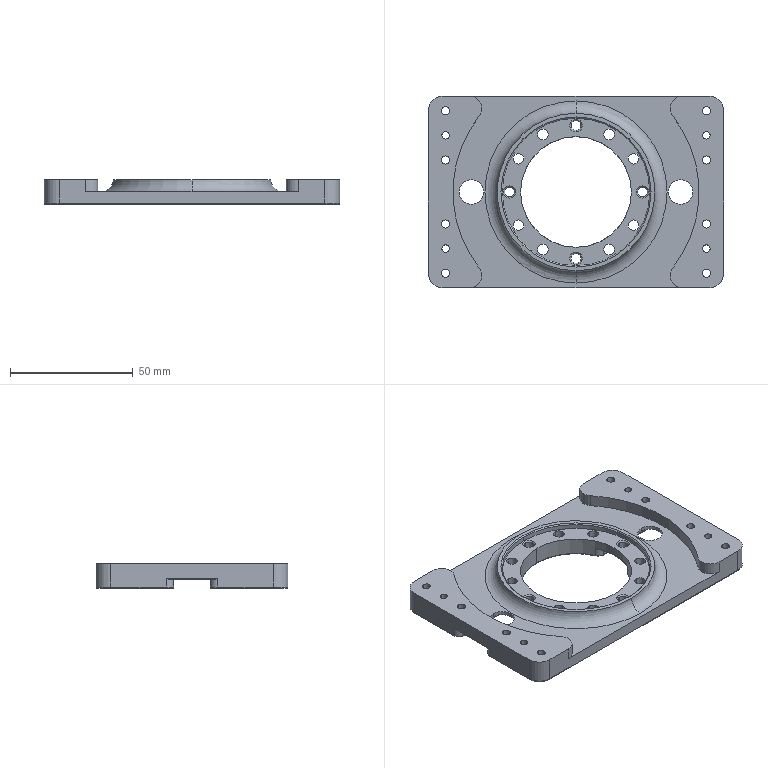NC program | NX | posted with a generic post | part box 120 x 78 x 10 mm
Lines 5880 to 6064 of 8419:
(FLOOR_WALL_COPY_COPY_COPY , TOOL : D6)
N11746 T12 M6
N11748 G54
N11750 G17 G0 G90 X-40.871 Y43.5 B0. C0. S9500 M3
N11752 G43 Z30. H12
N11754 Z-3.9
N11756 G94 G1 Z-4.9 F1000.
N11758 Y41.96
N11760 X-40.915 Y41.991
N11762 X-40.967 Y42.005
N11764 X-41.021 Y42.
N11766 X41.021 F1500.
N11768 G3 X36.675 Y39.089 R8.3
N11770 G1 X9.801
N11772 G2 X17.753 Y36.178 R40.299
N11774 G1 X35.223
N11776 G3 X34.964 Y33.267 R8.3
N11778 G1 X22.745
N11780 G2 X26.506 Y30.356 R40.299
N11782 G1 X35.775
N11784 G3 X36.708 Y28.869 R8.3
N11786 G2 X37.785 Y27.444 R46.7
N11788 G1 X29.51
N11790 G2 X31.971 Y24.533 R40.299
N11792 G1 X39.737
N11794 G2 X41.393 Y21.622 R46.7
N11796 G1 X34.007
N11798 G2 X35.692 Y18.711 R40.299
N11800 G1 X42.788
N11802 G2 X43.946 Y15.8 R46.7
N11804 G1 X37.072
N11806 G2 X38.182 Y12.889 R40.299
N11808 G1 X44.886
N11810 G2 X45.622 Y9.978 R46.7
N11812 G1 X39.044
N11814 G2 X39.675 Y7.067 R40.299
N11816 G1 X46.162
N11818 G2 X46.515 Y4.156 R46.7
N11820 G1 X40.084
N11822 G2 X40.28 Y1.244 R40.299
N11824 G1 X46.683
N11826 G2 X46.67 Y-1.667 R46.7
N11828 G1 X40.265
N11830 G2 X40.038 Y-4.578 R40.299
N11832 G1 X46.475
N11834 G2 X46.096 Y-7.489 R46.7
N11836 G1 X39.597
N11838 G2 X38.934 Y-10.4 R40.299
N11840 G1 X45.527
N11842 G2 X44.763 Y-13.311 R46.7
N11844 G1 X38.037
N11846 G2 X36.89 Y-16.222 R40.299
N11848 G1 X43.792
N11850 G2 X42.601 Y-19.133 R46.7
N11852 G1 X35.467
N11854 G2 X33.735 Y-22.044 R40.299
N11856 G1 X41.17
N11858 G2 X39.473 Y-24.956 R46.7
N11860 G1 X31.642
N11862 G2 X29.111 Y-27.867 R40.299
N11864 G1 X37.475
N11866 G2 X36.708 Y-28.869 R46.7
N11868 G3 X35.583 Y-30.778 R8.3
N11870 G1 X26.014
N11872 G2 X22.115 Y-33.689 R40.299
N11874 G1 X34.938
N11876 G3 X35.35 Y-36.6 R8.3
N11878 G1 X16.866
N11880 G2 X7.93 Y-39.511 R40.299
N11882 G1 X37.026
N11884 G3 X36.456 Y-39.322 R0.6
N11886 G1 Y-43.5
N11888 Z-3.9
N11890 G0 Z30.
N11892 X9.801 Y39.089
N11894 Z-3.9
N11896 G1 Z-4.9 F1000.
N11898 G3 X-9.801 Y39.089 R40.299
N11900 G1 X-36.675 F1500.
N11902 G2 X-35.223 Y36.178 R8.3
N11904 G1 X-17.753
N11906 G3 X-22.745 Y33.267 R40.299
N11908 G1 X-34.964
N11910 G2 X-35.775 Y30.356 R8.3
N11912 G1 X-26.506
N11914 G3 X-29.51 Y27.444 R40.299
N11916 G1 X-37.785
N11918 G3 X-39.737 Y24.533 R46.7
N11920 G1 X-31.971
N11922 G3 X-34.007 Y21.622 R40.299
N11924 G1 X-41.393
N11926 G3 X-42.788 Y18.711 R46.7
N11928 G1 X-35.692
N11930 G3 X-37.072 Y15.8 R40.299
N11932 G1 X-43.946
N11934 G3 X-44.886 Y12.889 R46.7
N11936 G1 X-38.182
N11938 G3 X-39.044 Y9.978 R40.299
N11940 G1 X-45.622
N11942 G3 X-46.162 Y7.067 R46.7
N11944 G1 X-39.675
N11946 G3 X-40.084 Y4.156 R40.299
N11948 G1 X-46.515
N11950 G3 X-46.683 Y1.244 R46.7
N11952 G1 X-40.28
N11954 G3 X-40.265 Y-1.667 R40.299
N11956 G1 X-46.67
N11958 G3 X-46.475 Y-4.578 R46.7
N11960 G1 X-40.038
N11962 G3 X-39.597 Y-7.489 R40.299
N11964 G1 X-46.096
N11966 G3 X-45.527 Y-10.4 R46.7
N11968 G1 X-38.934
N11970 G3 X-38.037 Y-13.311 R40.299
N11972 G1 X-44.763
N11974 G3 X-43.792 Y-16.222 R46.7
N11976 G1 X-36.89
N11978 G3 X-35.467 Y-19.133 R40.299
N11980 G1 X-42.601
N11982 G3 X-41.17 Y-22.044 R46.7
N11984 G1 X-33.735
N11986 G3 X-31.642 Y-24.956 R40.299
N11988 G1 X-39.473
N11990 G3 X-37.475 Y-27.867 R46.7
N11992 G1 X-29.111
N11994 G3 X-26.014 Y-30.778 R40.299
N11996 G1 X-35.583
N11998 G2 X-34.938 Y-33.689 R8.3
N12000 G1 X-22.115
N12002 G3 X-16.866 Y-36.6 R40.299
N12004 G1 X-35.35
N12006 G2 X-37.026 Y-39.511 R8.3
N12008 G1 X-7.93
N12010 G3 X-8.494 Y-39.716 R0.6
N12012 G1 Y-43.5
N12014 Z-3.9
N12016 G0 Z30.
N12018 X39.808
N12020 Z-3.9
N12022 G1 Z-4.9 F1000.
N12024 X40.501 Y-42.3
N12026 G2 X41.021 Y-42. R0.6
N12028 G1 X-4.973 F1500.
N12030 G2 X-5.493 Y-41.7 R0.6
N12032 G1 Y-43.5
N12034 Z-3.9
N12036 G0 Z30.
N12038 X43.943
N12040 Z-3.9
N12042 G1 Z-4.9 F1000.
N12044 X43.336 Y-42.316
N12046 G3 X42.832 Y-41.99 R0.6
N12048 G2 X36.944 Y-29.055 R8. F1500.
N12050 G3 X36.944 Y29.055 R47.
N12052 G2 X42.832 Y41.99 R8.
N12054 G3 X43.336 Y42.316 R0.6
N12056 G1 X43.943 Y43.5
N12058 Z-3.9
N12060 G0 Z30.
N12062 X-43.943
N12064 Z-3.9
N12066 G1 Z-4.9 F1000.
N12068 X-43.336 Y42.316
N12070 G3 X-42.832 Y41.99 R0.6
N12072 G2 X-36.944 Y29.055 R8. F1500.
N12074 G3 X-36.944 Y-29.055 R47.
N12076 G2 X-42.832 Y-41.99 R8.
N12078 G3 X-43.336 Y-42.316 R0.6
N12080 G1 X-43.943 Y-43.5
N12082 Z-3.9
N12084 G0 Z30.
N12086 X0.52
N12088 Z-3.9
N12090 G1 Z-4.9 F1000.
N12092 Y-40.299
N12094 G3 X0. Y-39.999 R0.6
N12096 G2 X-39.999 Y0. R39.999 F1500.
N12098 X0. Y-39.999 R-39.999
N12100 G3 X-0.52 Y-40.299 R0.6
N12102 G1 X-1.373 Y-41.776
N12104 Z-3.9
N12106 G0 Z30.
N12108 M5